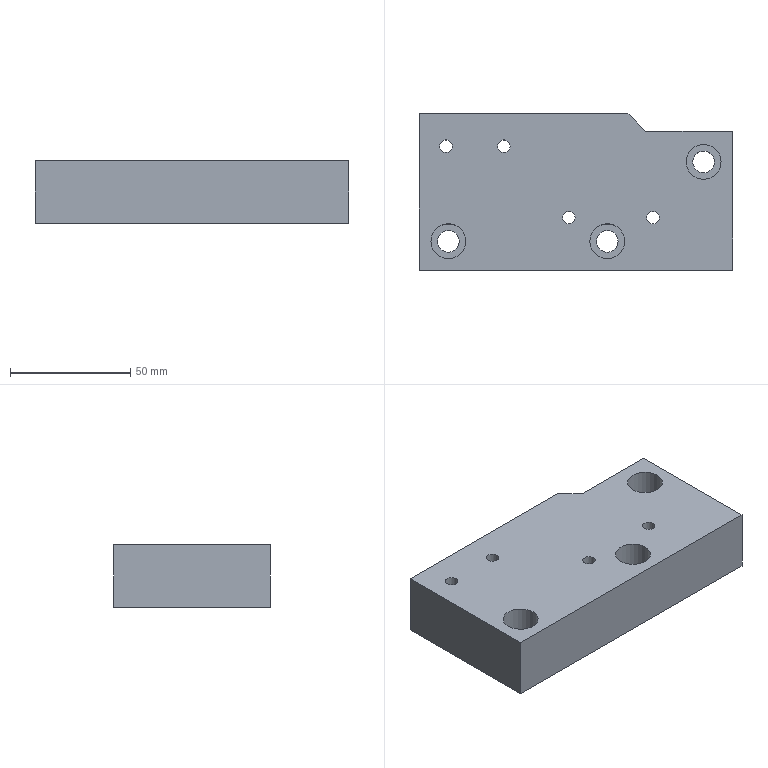Part | STEP file | lll_id678_x_t | 1 solid | 21 faces | box 130 x 65 x 26 mm | volume 201593 mm3 | plane 11 | cylinder 10 | commonest cylinder face diameters 5.206 x4 9.009 x3 14.508 x3
STEP:
#1=CARTESIAN_POINT('',(321.902,-180.325,-12.));
#2=VERTEX_POINT('',#1);
#3=CARTESIAN_POINT('',(324.505,-180.325,-12.));
#4=DIRECTION('',(0.,0.,-1.));
#5=DIRECTION('',(-1.,0.,0.));
#6=AXIS2_PLACEMENT_3D('',#3,#4,#5);
#7=CIRCLE('',#6,2.603);
#8=EDGE_CURVE('',#2,#2,#7,.T.);
#9=ORIENTED_EDGE('',*,*,#8,.T.);
#10=EDGE_LOOP('',(#9));
#11=FACE_BOUND('',#10,.T.);
#12=CARTESIAN_POINT('',(356.42,-144.5,-12.));
#13=VERTEX_POINT('',#12);
#14=CARTESIAN_POINT('',(349.095,-137.175,-12.));
#15=VERTEX_POINT('',#14);
#16=CARTESIAN_POINT('',(367.15,-155.231,-12.));
#17=DIRECTION('',(-0.7071,0.7071,0.));
#18=VECTOR('',#17,1.);
#19=LINE('',#16,#18);
#20=EDGE_CURVE('',#13,#15,#19,.T.);
#21=ORIENTED_EDGE('',*,*,#20,.T.);
#22=CARTESIAN_POINT('',(262.505,-137.175,-12.));
#23=VERTEX_POINT('',#22);
#24=CARTESIAN_POINT('',(317.505,-137.175,-12.));
#25=DIRECTION('',(-1.,0.,0.));
#26=VECTOR('',#25,1.);
#27=LINE('',#24,#26);
#28=EDGE_CURVE('',#15,#23,#27,.T.);
#29=ORIENTED_EDGE('',*,*,#28,.T.);
#30=CARTESIAN_POINT('',(262.505,-202.175,-12.));
#31=VERTEX_POINT('',#30);
#32=CARTESIAN_POINT('',(262.505,-159.675,-12.));
#33=DIRECTION('',(0.,-1.,0.));
#34=VECTOR('',#33,1.);
#35=LINE('',#32,#34);
#36=EDGE_CURVE('',#23,#31,#35,.T.);
#37=ORIENTED_EDGE('',*,*,#36,.T.);
#38=CARTESIAN_POINT('',(392.505,-202.175,-12.));
#39=VERTEX_POINT('',#38);
#40=CARTESIAN_POINT('',(317.505,-202.175,-12.));
#41=DIRECTION('',(1.,0.,0.));
#42=VECTOR('',#41,1.);
#43=LINE('',#40,#42);
#44=EDGE_CURVE('',#31,#39,#43,.T.);
#45=ORIENTED_EDGE('',*,*,#44,.T.);
#46=CARTESIAN_POINT('',(392.505,-144.5,-12.));
#47=VERTEX_POINT('',#46);
#48=CARTESIAN_POINT('',(392.505,-159.675,-12.));
#49=DIRECTION('',(0.,1.,0.));
#50=VECTOR('',#49,1.);
#51=LINE('',#48,#50);
#52=EDGE_CURVE('',#39,#47,#51,.T.);
#53=ORIENTED_EDGE('',*,*,#52,.T.);
#54=CARTESIAN_POINT('',(317.505,-144.5,-12.));
#55=DIRECTION('',(-1.,0.,0.));
#56=VECTOR('',#55,1.);
#57=LINE('',#54,#56);
#58=EDGE_CURVE('',#47,#13,#57,.T.);
#59=ORIENTED_EDGE('',*,*,#58,.T.);
#60=EDGE_LOOP('',(#21,#29,#37,#45,#53,#59));
#61=FACE_BOUND('',#60,.T.);
#62=CARTESIAN_POINT('',(270.902,-150.675,-12.));
#63=VERTEX_POINT('',#62);
#64=CARTESIAN_POINT('',(273.505,-150.675,-12.));
#65=DIRECTION('',(0.,0.,1.));
#66=DIRECTION('',(-1.,0.,0.));
#67=AXIS2_PLACEMENT_3D('',#64,#65,#66);
#68=CIRCLE('',#67,2.603);
#69=EDGE_CURVE('',#63,#63,#68,.T.);
#70=ORIENTED_EDGE('',*,*,#69,.F.);
#71=EDGE_LOOP('',(#70));
#72=FACE_BOUND('',#71,.T.);
#73=CARTESIAN_POINT('',(333.251,-190.175,-12.));
#74=VERTEX_POINT('',#73);
#75=CARTESIAN_POINT('',(340.505,-190.175,-12.));
#76=DIRECTION('',(0.,0.,1.));
#77=DIRECTION('',(-1.,0.,0.));
#78=AXIS2_PLACEMENT_3D('',#75,#76,#77);
#79=CIRCLE('',#78,7.254);
#80=EDGE_CURVE('',#74,#74,#79,.T.);
#81=ORIENTED_EDGE('',*,*,#80,.F.);
#82=EDGE_LOOP('',(#81));
#83=FACE_BOUND('',#82,.T.);
#84=CARTESIAN_POINT('',(267.251,-190.175,-12.));
#85=VERTEX_POINT('',#84);
#86=CARTESIAN_POINT('',(274.505,-190.175,-12.));
#87=DIRECTION('',(0.,0.,1.));
#88=DIRECTION('',(-1.,0.,0.));
#89=AXIS2_PLACEMENT_3D('',#86,#87,#88);
#90=CIRCLE('',#89,7.254);
#91=EDGE_CURVE('',#85,#85,#90,.T.);
#92=ORIENTED_EDGE('',*,*,#91,.F.);
#93=EDGE_LOOP('',(#92));
#94=FACE_BOUND('',#93,.T.);
#95=CARTESIAN_POINT('',(373.251,-157.175,-12.));
#96=VERTEX_POINT('',#95);
#97=CARTESIAN_POINT('',(380.505,-157.175,-12.));
#98=DIRECTION('',(0.,0.,1.));
#99=DIRECTION('',(-1.,0.,0.));
#100=AXIS2_PLACEMENT_3D('',#97,#98,#99);
#101=CIRCLE('',#100,7.254);
#102=EDGE_CURVE('',#96,#96,#101,.T.);
#103=ORIENTED_EDGE('',*,*,#102,.F.);
#104=EDGE_LOOP('',(#103));
#105=FACE_BOUND('',#104,.T.);
#106=CARTESIAN_POINT('',(294.902,-150.675,-12.));
#107=VERTEX_POINT('',#106);
#108=CARTESIAN_POINT('',(297.505,-150.675,-12.));
#109=DIRECTION('',(0.,0.,1.));
#110=DIRECTION('',(-1.,0.,0.));
#111=AXIS2_PLACEMENT_3D('',#108,#109,#110);
#112=CIRCLE('',#111,2.603);
#113=EDGE_CURVE('',#107,#107,#112,.T.);
#114=ORIENTED_EDGE('',*,*,#113,.F.);
#115=EDGE_LOOP('',(#114));
#116=FACE_BOUND('',#115,.T.);
#117=CARTESIAN_POINT('',(356.902,-180.325,-12.));
#118=VERTEX_POINT('',#117);
#119=CARTESIAN_POINT('',(359.505,-180.325,-12.));
#120=DIRECTION('',(0.,0.,-1.));
#121=DIRECTION('',(-1.,0.,0.));
#122=AXIS2_PLACEMENT_3D('',#119,#120,#121);
#123=CIRCLE('',#122,2.603);
#124=EDGE_CURVE('',#118,#118,#123,.T.);
#125=ORIENTED_EDGE('',*,*,#124,.T.);
#126=EDGE_LOOP('',(#125));
#127=FACE_BOUND('',#126,.T.);
#128=CARTESIAN_POINT('',(317.505,-159.675,-12.));
#129=DIRECTION('',(0.,0.,1.));
#130=DIRECTION('',(-1.,0.,0.));
#131=AXIS2_PLACEMENT_3D('',#128,#129,#130);
#132=PLANE('',#131);
#133=ADVANCED_FACE('',(#11,#61,#72,#83,#94,#105,#116,#127),#132,.T.);
#134=CARTESIAN_POINT('',(262.505,-137.175,-38.));
#135=VERTEX_POINT('',#134);
#136=CARTESIAN_POINT('',(349.095,-137.175,-38.));
#137=VERTEX_POINT('',#136);
#138=CARTESIAN_POINT('',(317.505,-137.175,-38.));
#139=DIRECTION('',(1.,0.,0.));
#140=VECTOR('',#139,1.);
#141=LINE('',#138,#140);
#142=EDGE_CURVE('',#135,#137,#141,.T.);
#143=ORIENTED_EDGE('',*,*,#142,.F.);
#144=CARTESIAN_POINT('',(262.505,-137.175,-38.));
#145=DIRECTION('',(0.,0.,1.));
#146=VECTOR('',#145,1.);
#147=LINE('',#144,#146);
#148=EDGE_CURVE('',#135,#23,#147,.T.);
#149=ORIENTED_EDGE('',*,*,#148,.T.);
#150=ORIENTED_EDGE('',*,*,#28,.F.);
#151=CARTESIAN_POINT('',(349.095,-137.175,-38.));
#152=DIRECTION('',(0.,0.,-1.));
#153=VECTOR('',#152,1.);
#154=LINE('',#151,#153);
#155=EDGE_CURVE('',#15,#137,#154,.T.);
#156=ORIENTED_EDGE('',*,*,#155,.T.);
#157=EDGE_LOOP('',(#143,#149,#150,#156));
#158=FACE_OUTER_BOUND('',#157,.T.);
#159=CARTESIAN_POINT('',(317.505,-137.175,-38.));
#160=DIRECTION('',(0.,1.,0.));
#161=DIRECTION('',(0.,0.,1.));
#162=AXIS2_PLACEMENT_3D('',#159,#160,#161);
#163=PLANE('',#162);
#164=ADVANCED_FACE('',(#158),#163,.T.);
#165=ORIENTED_EDGE('',*,*,#148,.F.);
#166=CARTESIAN_POINT('',(262.505,-202.175,-38.));
#167=VERTEX_POINT('',#166);
#168=CARTESIAN_POINT('',(262.505,-159.675,-38.));
#169=DIRECTION('',(0.,1.,0.));
#170=VECTOR('',#169,1.);
#171=LINE('',#168,#170);
#172=EDGE_CURVE('',#167,#135,#171,.T.);
#173=ORIENTED_EDGE('',*,*,#172,.F.);
#174=CARTESIAN_POINT('',(262.505,-202.175,-38.));
#175=DIRECTION('',(0.,0.,1.));
#176=VECTOR('',#175,1.);
#177=LINE('',#174,#176);
#178=EDGE_CURVE('',#167,#31,#177,.T.);
#179=ORIENTED_EDGE('',*,*,#178,.T.);
#180=ORIENTED_EDGE('',*,*,#36,.F.);
#181=EDGE_LOOP('',(#165,#173,#179,#180));
#182=FACE_OUTER_BOUND('',#181,.T.);
#183=CARTESIAN_POINT('',(262.505,-159.675,-38.));
#184=DIRECTION('',(-1.,0.,0.));
#185=DIRECTION('',(0.,0.,-1.));
#186=AXIS2_PLACEMENT_3D('',#183,#184,#185);
#187=PLANE('',#186);
#188=ADVANCED_FACE('',(#182),#187,.T.);
#189=ORIENTED_EDGE('',*,*,#178,.F.);
#190=CARTESIAN_POINT('',(392.505,-202.175,-38.));
#191=VERTEX_POINT('',#190);
#192=CARTESIAN_POINT('',(317.505,-202.175,-38.));
#193=DIRECTION('',(-1.,0.,0.));
#194=VECTOR('',#193,1.);
#195=LINE('',#192,#194);
#196=EDGE_CURVE('',#191,#167,#195,.T.);
#197=ORIENTED_EDGE('',*,*,#196,.F.);
#198=CARTESIAN_POINT('',(392.505,-202.175,-38.));
#199=DIRECTION('',(0.,0.,1.));
#200=VECTOR('',#199,1.);
#201=LINE('',#198,#200);
#202=EDGE_CURVE('',#191,#39,#201,.T.);
#203=ORIENTED_EDGE('',*,*,#202,.T.);
#204=ORIENTED_EDGE('',*,*,#44,.F.);
#205=EDGE_LOOP('',(#189,#197,#203,#204));
#206=FACE_OUTER_BOUND('',#205,.T.);
#207=CARTESIAN_POINT('',(317.505,-202.175,-38.));
#208=DIRECTION('',(0.,-1.,0.));
#209=DIRECTION('',(0.,0.,-1.));
#210=AXIS2_PLACEMENT_3D('',#207,#208,#209);
#211=PLANE('',#210);
#212=ADVANCED_FACE('',(#206),#211,.T.);
#213=CARTESIAN_POINT('',(356.902,-180.325,-38.));
#214=VERTEX_POINT('',#213);
#215=CARTESIAN_POINT('',(359.505,-180.325,-38.));
#216=DIRECTION('',(0.,0.,-1.));
#217=DIRECTION('',(-1.,0.,0.));
#218=AXIS2_PLACEMENT_3D('',#215,#216,#217);
#219=CIRCLE('',#218,2.603);
#220=EDGE_CURVE('',#214,#214,#219,.T.);
#221=ORIENTED_EDGE('',*,*,#220,.F.);
#222=EDGE_LOOP('',(#221));
#223=FACE_BOUND('',#222,.T.);
#224=CARTESIAN_POINT('',(321.902,-180.325,-38.));
#225=VERTEX_POINT('',#224);
#226=CARTESIAN_POINT('',(324.505,-180.325,-38.));
#227=DIRECTION('',(0.,0.,-1.));
#228=DIRECTION('',(-1.,0.,0.));
#229=AXIS2_PLACEMENT_3D('',#226,#227,#228);
#230=CIRCLE('',#229,2.603);
#231=EDGE_CURVE('',#225,#225,#230,.T.);
#232=ORIENTED_EDGE('',*,*,#231,.F.);
#233=EDGE_LOOP('',(#232));
#234=FACE_BOUND('',#233,.T.);
#235=CARTESIAN_POINT('',(356.42,-144.5,-38.));
#236=VERTEX_POINT('',#235);
#237=CARTESIAN_POINT('',(392.505,-144.5,-38.));
#238=VERTEX_POINT('',#237);
#239=CARTESIAN_POINT('',(317.505,-144.5,-38.));
#240=DIRECTION('',(1.,0.,0.));
#241=VECTOR('',#240,1.);
#242=LINE('',#239,#241);
#243=EDGE_CURVE('',#236,#238,#242,.T.);
#244=ORIENTED_EDGE('',*,*,#243,.T.);
#245=CARTESIAN_POINT('',(392.505,-159.675,-38.));
#246=DIRECTION('',(0.,-1.,0.));
#247=VECTOR('',#246,1.);
#248=LINE('',#245,#247);
#249=EDGE_CURVE('',#238,#191,#248,.T.);
#250=ORIENTED_EDGE('',*,*,#249,.T.);
#251=ORIENTED_EDGE('',*,*,#196,.T.);
#252=ORIENTED_EDGE('',*,*,#172,.T.);
#253=ORIENTED_EDGE('',*,*,#142,.T.);
#254=CARTESIAN_POINT('',(335.56,-123.641,-38.));
#255=DIRECTION('',(-0.7071,0.7071,0.));
#256=VECTOR('',#255,1.);
#257=LINE('',#254,#256);
#258=EDGE_CURVE('',#236,#137,#257,.T.);
#259=ORIENTED_EDGE('',*,*,#258,.F.);
#260=EDGE_LOOP('',(#244,#250,#251,#252,#253,#259));
#261=FACE_BOUND('',#260,.T.);
#262=CARTESIAN_POINT('',(294.902,-150.675,-38.));
#263=VERTEX_POINT('',#262);
#264=CARTESIAN_POINT('',(297.505,-150.675,-38.));
#265=DIRECTION('',(0.,0.,1.));
#266=DIRECTION('',(-1.,0.,0.));
#267=AXIS2_PLACEMENT_3D('',#264,#265,#266);
#268=CIRCLE('',#267,2.603);
#269=EDGE_CURVE('',#263,#263,#268,.T.);
#270=ORIENTED_EDGE('',*,*,#269,.T.);
#271=EDGE_LOOP('',(#270));
#272=FACE_BOUND('',#271,.T.);
#273=CARTESIAN_POINT('',(270.902,-150.675,-38.));
#274=VERTEX_POINT('',#273);
#275=CARTESIAN_POINT('',(273.505,-150.675,-38.));
#276=DIRECTION('',(0.,0.,1.));
#277=DIRECTION('',(-1.,0.,0.));
#278=AXIS2_PLACEMENT_3D('',#275,#276,#277);
#279=CIRCLE('',#278,2.603);
#280=EDGE_CURVE('',#274,#274,#279,.T.);
#281=ORIENTED_EDGE('',*,*,#280,.T.);
#282=EDGE_LOOP('',(#281));
#283=FACE_BOUND('',#282,.T.);
#284=CARTESIAN_POINT('',(376.,-157.175,-38.));
#285=VERTEX_POINT('',#284);
#286=CARTESIAN_POINT('',(380.505,-157.175,-38.));
#287=DIRECTION('',(0.,0.,1.));
#288=DIRECTION('',(-1.,0.,0.));
#289=AXIS2_PLACEMENT_3D('',#286,#287,#288);
#290=CIRCLE('',#289,4.505);
#291=EDGE_CURVE('',#285,#285,#290,.T.);
#292=ORIENTED_EDGE('',*,*,#291,.T.);
#293=EDGE_LOOP('',(#292));
#294=FACE_BOUND('',#293,.T.);
#295=CARTESIAN_POINT('',(336.,-190.175,-38.));
#296=VERTEX_POINT('',#295);
#297=CARTESIAN_POINT('',(340.505,-190.175,-38.));
#298=DIRECTION('',(0.,0.,1.));
#299=DIRECTION('',(-1.,0.,0.));
#300=AXIS2_PLACEMENT_3D('',#297,#298,#299);
#301=CIRCLE('',#300,4.505);
#302=EDGE_CURVE('',#296,#296,#301,.T.);
#303=ORIENTED_EDGE('',*,*,#302,.T.);
#304=EDGE_LOOP('',(#303));
#305=FACE_BOUND('',#304,.T.);
#306=CARTESIAN_POINT('',(270.,-190.175,-38.));
#307=VERTEX_POINT('',#306);
#308=CARTESIAN_POINT('',(274.505,-190.175,-38.));
#309=DIRECTION('',(0.,0.,1.));
#310=DIRECTION('',(-1.,0.,0.));
#311=AXIS2_PLACEMENT_3D('',#308,#309,#310);
#312=CIRCLE('',#311,4.505);
#313=EDGE_CURVE('',#307,#307,#312,.T.);
#314=ORIENTED_EDGE('',*,*,#313,.T.);
#315=EDGE_LOOP('',(#314));
#316=FACE_BOUND('',#315,.T.);
#317=CARTESIAN_POINT('',(317.505,-159.675,-38.));
#318=DIRECTION('',(0.,0.,-1.));
#319=DIRECTION('',(1.,0.,0.));
#320=AXIS2_PLACEMENT_3D('',#317,#318,#319);
#321=PLANE('',#320);
#322=ADVANCED_FACE('',(#223,#234,#261,#272,#283,#294,#305,#316),#321,.T.);
#323=CARTESIAN_POINT('',(392.505,-144.5,-38.));
#324=DIRECTION('',(0.,0.,1.));
#325=VECTOR('',#324,1.);
#326=LINE('',#323,#325);
#327=EDGE_CURVE('',#238,#47,#326,.T.);
#328=ORIENTED_EDGE('',*,*,#327,.T.);
#329=ORIENTED_EDGE('',*,*,#52,.F.);
#330=ORIENTED_EDGE('',*,*,#202,.F.);
#331=ORIENTED_EDGE('',*,*,#249,.F.);
#332=EDGE_LOOP('',(#328,#329,#330,#331));
#333=FACE_OUTER_BOUND('',#332,.T.);
#334=CARTESIAN_POINT('',(392.505,-159.675,-38.));
#335=DIRECTION('',(1.,0.,0.));
#336=DIRECTION('',(0.,0.,1.));
#337=AXIS2_PLACEMENT_3D('',#334,#335,#336);
#338=PLANE('',#337);
#339=ADVANCED_FACE('',(#333),#338,.T.);
#340=ORIENTED_EDGE('',*,*,#313,.F.);
#341=EDGE_LOOP('',(#340));
#342=FACE_BOUND('',#341,.T.);
#343=CARTESIAN_POINT('',(270.,-190.175,-23.));
#344=VERTEX_POINT('',#343);
#345=CARTESIAN_POINT('',(274.505,-190.175,-23.));
#346=DIRECTION('',(0.,0.,1.));
#347=DIRECTION('',(-1.,0.,0.));
#348=AXIS2_PLACEMENT_3D('',#345,#346,#347);
#349=CIRCLE('',#348,4.505);
#350=EDGE_CURVE('',#344,#344,#349,.T.);
#351=ORIENTED_EDGE('',*,*,#350,.T.);
#352=EDGE_LOOP('',(#351));
#353=FACE_BOUND('',#352,.T.);
#354=CARTESIAN_POINT('',(274.505,-190.175,-10.));
#355=DIRECTION('',(0.,0.,-1.));
#356=DIRECTION('',(1.,0.,0.));
#357=AXIS2_PLACEMENT_3D('',#354,#355,#356);
#358=CYLINDRICAL_SURFACE('',#357,4.505);
#359=ADVANCED_FACE('',(#342,#353),#358,.F.);
#360=ORIENTED_EDGE('',*,*,#350,.F.);
#361=EDGE_LOOP('',(#360));
#362=FACE_BOUND('',#361,.T.);
#363=CARTESIAN_POINT('',(267.251,-190.175,-23.));
#364=VERTEX_POINT('',#363);
#365=CARTESIAN_POINT('',(274.505,-190.175,-23.));
#366=DIRECTION('',(0.,0.,1.));
#367=DIRECTION('',(-1.,0.,0.));
#368=AXIS2_PLACEMENT_3D('',#365,#366,#367);
#369=CIRCLE('',#368,7.254);
#370=EDGE_CURVE('',#364,#364,#369,.T.);
#371=ORIENTED_EDGE('',*,*,#370,.T.);
#372=EDGE_LOOP('',(#371));
#373=FACE_BOUND('',#372,.T.);
#374=CARTESIAN_POINT('',(274.505,-190.175,-23.));
#375=DIRECTION('',(0.,0.,-1.));
#376=DIRECTION('',(1.,0.,0.));
#377=AXIS2_PLACEMENT_3D('',#374,#375,#376);
#378=PLANE('',#377);
#379=ADVANCED_FACE('',(#362,#373),#378,.F.);
#380=ORIENTED_EDGE('',*,*,#370,.F.);
#381=EDGE_LOOP('',(#380));
#382=FACE_BOUND('',#381,.T.);
#383=ORIENTED_EDGE('',*,*,#91,.T.);
#384=EDGE_LOOP('',(#383));
#385=FACE_BOUND('',#384,.T.);
#386=CARTESIAN_POINT('',(274.505,-190.175,-12.));
#387=DIRECTION('',(0.,0.,-1.));
#388=DIRECTION('',(1.,0.,0.));
#389=AXIS2_PLACEMENT_3D('',#386,#387,#388);
#390=CYLINDRICAL_SURFACE('',#389,7.254);
#391=ADVANCED_FACE('',(#382,#385),#390,.F.);
#392=ORIENTED_EDGE('',*,*,#302,.F.);
#393=EDGE_LOOP('',(#392));
#394=FACE_BOUND('',#393,.T.);
#395=CARTESIAN_POINT('',(336.,-190.175,-23.));
#396=VERTEX_POINT('',#395);
#397=CARTESIAN_POINT('',(340.505,-190.175,-23.));
#398=DIRECTION('',(0.,0.,1.));
#399=DIRECTION('',(-1.,0.,0.));
#400=AXIS2_PLACEMENT_3D('',#397,#398,#399);
#401=CIRCLE('',#400,4.505);
#402=EDGE_CURVE('',#396,#396,#401,.T.);
#403=ORIENTED_EDGE('',*,*,#402,.T.);
#404=EDGE_LOOP('',(#403));
#405=FACE_BOUND('',#404,.T.);
#406=CARTESIAN_POINT('',(340.505,-190.175,-10.));
#407=DIRECTION('',(0.,0.,-1.));
#408=DIRECTION('',(1.,0.,0.));
#409=AXIS2_PLACEMENT_3D('',#406,#407,#408);
#410=CYLINDRICAL_SURFACE('',#409,4.505);
#411=ADVANCED_FACE('',(#394,#405),#410,.F.);
#412=ORIENTED_EDGE('',*,*,#402,.F.);
#413=EDGE_LOOP('',(#412));
#414=FACE_BOUND('',#413,.T.);
#415=CARTESIAN_POINT('',(333.251,-190.175,-23.));
#416=VERTEX_POINT('',#415);
#417=CARTESIAN_POINT('',(340.505,-190.175,-23.));
#418=DIRECTION('',(0.,0.,1.));
#419=DIRECTION('',(-1.,0.,0.));
#420=AXIS2_PLACEMENT_3D('',#417,#418,#419);
#421=CIRCLE('',#420,7.254);
#422=EDGE_CURVE('',#416,#416,#421,.T.);
#423=ORIENTED_EDGE('',*,*,#422,.T.);
#424=EDGE_LOOP('',(#423));
#425=FACE_BOUND('',#424,.T.);
#426=CARTESIAN_POINT('',(340.505,-190.175,-23.));
#427=DIRECTION('',(0.,0.,-1.));
#428=DIRECTION('',(1.,0.,0.));
#429=AXIS2_PLACEMENT_3D('',#426,#427,#428);
#430=PLANE('',#429);
#431=ADVANCED_FACE('',(#414,#425),#430,.F.);
#432=ORIENTED_EDGE('',*,*,#422,.F.);
#433=EDGE_LOOP('',(#432));
#434=FACE_BOUND('',#433,.T.);
#435=ORIENTED_EDGE('',*,*,#80,.T.);
#436=EDGE_LOOP('',(#435));
#437=FACE_BOUND('',#436,.T.);
#438=CARTESIAN_POINT('',(340.505,-190.175,-12.));
#439=DIRECTION('',(0.,0.,-1.));
#440=DIRECTION('',(1.,0.,0.));
#441=AXIS2_PLACEMENT_3D('',#438,#439,#440);
#442=CYLINDRICAL_SURFACE('',#441,7.254);
#443=ADVANCED_FACE('',(#434,#437),#442,.F.);
#444=ORIENTED_EDGE('',*,*,#291,.F.);
#445=EDGE_LOOP('',(#444));
#446=FACE_BOUND('',#445,.T.);
#447=CARTESIAN_POINT('',(376.,-157.175,-23.));
#448=VERTEX_POINT('',#447);
#449=CARTESIAN_POINT('',(380.505,-157.175,-23.));
#450=DIRECTION('',(0.,0.,1.));
#451=DIRECTION('',(-1.,0.,0.));
#452=AXIS2_PLACEMENT_3D('',#449,#450,#451);
#453=CIRCLE('',#452,4.505);
#454=EDGE_CURVE('',#448,#448,#453,.T.);
#455=ORIENTED_EDGE('',*,*,#454,.T.);
#456=EDGE_LOOP('',(#455));
#457=FACE_BOUND('',#456,.T.);
#458=CARTESIAN_POINT('',(380.505,-157.175,-10.));
#459=DIRECTION('',(0.,0.,-1.));
#460=DIRECTION('',(1.,0.,0.));
#461=AXIS2_PLACEMENT_3D('',#458,#459,#460);
#462=CYLINDRICAL_SURFACE('',#461,4.505);
#463=ADVANCED_FACE('',(#446,#457),#462,.F.);
#464=ORIENTED_EDGE('',*,*,#454,.F.);
#465=EDGE_LOOP('',(#464));
#466=FACE_BOUND('',#465,.T.);
#467=CARTESIAN_POINT('',(373.251,-157.175,-23.));
#468=VERTEX_POINT('',#467);
#469=CARTESIAN_POINT('',(380.505,-157.175,-23.));
#470=DIRECTION('',(0.,0.,1.));
#471=DIRECTION('',(-1.,0.,0.));
#472=AXIS2_PLACEMENT_3D('',#469,#470,#471);
#473=CIRCLE('',#472,7.254);
#474=EDGE_CURVE('',#468,#468,#473,.T.);
#475=ORIENTED_EDGE('',*,*,#474,.T.);
#476=EDGE_LOOP('',(#475));
#477=FACE_BOUND('',#476,.T.);
#478=CARTESIAN_POINT('',(380.505,-157.175,-23.));
#479=DIRECTION('',(0.,0.,-1.));
#480=DIRECTION('',(1.,0.,0.));
#481=AXIS2_PLACEMENT_3D('',#478,#479,#480);
#482=PLANE('',#481);
#483=ADVANCED_FACE('',(#466,#477),#482,.F.);
#484=ORIENTED_EDGE('',*,*,#474,.F.);
#485=EDGE_LOOP('',(#484));
#486=FACE_BOUND('',#485,.T.);
#487=ORIENTED_EDGE('',*,*,#102,.T.);
#488=EDGE_LOOP('',(#487));
#489=FACE_BOUND('',#488,.T.);
#490=CARTESIAN_POINT('',(380.505,-157.175,-12.));
#491=DIRECTION('',(0.,0.,-1.));
#492=DIRECTION('',(1.,0.,0.));
#493=AXIS2_PLACEMENT_3D('',#490,#491,#492);
#494=CYLINDRICAL_SURFACE('',#493,7.254);
#495=ADVANCED_FACE('',(#486,#489),#494,.F.);
#496=ORIENTED_EDGE('',*,*,#280,.F.);
#497=EDGE_LOOP('',(#496));
#498=FACE_BOUND('',#497,.T.);
#499=ORIENTED_EDGE('',*,*,#69,.T.);
#500=EDGE_LOOP('',(#499));
#501=FACE_BOUND('',#500,.T.);
#502=CARTESIAN_POINT('',(273.505,-150.675,-12.));
#503=DIRECTION('',(0.,0.,-1.));
#504=DIRECTION('',(1.,0.,0.));
#505=AXIS2_PLACEMENT_3D('',#502,#503,#504);
#506=CYLINDRICAL_SURFACE('',#505,2.603);
#507=ADVANCED_FACE('',(#498,#501),#506,.F.);
#508=ORIENTED_EDGE('',*,*,#269,.F.);
#509=EDGE_LOOP('',(#508));
#510=FACE_BOUND('',#509,.T.);
#511=ORIENTED_EDGE('',*,*,#113,.T.);
#512=EDGE_LOOP('',(#511));
#513=FACE_BOUND('',#512,.T.);
#514=CARTESIAN_POINT('',(297.505,-150.675,-12.));
#515=DIRECTION('',(0.,0.,-1.));
#516=DIRECTION('',(1.,0.,0.));
#517=AXIS2_PLACEMENT_3D('',#514,#515,#516);
#518=CYLINDRICAL_SURFACE('',#517,2.603);
#519=ADVANCED_FACE('',(#510,#513),#518,.F.);
#520=ORIENTED_EDGE('',*,*,#258,.T.);
#521=ORIENTED_EDGE('',*,*,#155,.F.);
#522=ORIENTED_EDGE('',*,*,#20,.F.);
#523=CARTESIAN_POINT('',(356.42,-144.5,-20.));
#524=DIRECTION('',(0.,0.,-1.));
#525=VECTOR('',#524,1.);
#526=LINE('',#523,#525);
#527=EDGE_CURVE('',#13,#236,#526,.T.);
#528=ORIENTED_EDGE('',*,*,#527,.T.);
#529=EDGE_LOOP('',(#520,#521,#522,#528));
#530=FACE_OUTER_BOUND('',#529,.T.);
#531=CARTESIAN_POINT('',(335.56,-123.641,-20.));
#532=DIRECTION('',(-0.7071,-0.7071,0.));
#533=DIRECTION('',(0.,0.,-1.));
#534=AXIS2_PLACEMENT_3D('',#531,#532,#533);
#535=PLANE('',#534);
#536=ADVANCED_FACE('',(#530),#535,.F.);
#537=ORIENTED_EDGE('',*,*,#58,.F.);
#538=ORIENTED_EDGE('',*,*,#327,.F.);
#539=ORIENTED_EDGE('',*,*,#243,.F.);
#540=ORIENTED_EDGE('',*,*,#527,.F.);
#541=EDGE_LOOP('',(#537,#538,#539,#540));
#542=FACE_OUTER_BOUND('',#541,.T.);
#543=CARTESIAN_POINT('',(383.42,-144.5,-20.));
#544=DIRECTION('',(0.,-1.,0.));
#545=DIRECTION('',(0.,0.,-1.));
#546=AXIS2_PLACEMENT_3D('',#543,#544,#545);
#547=PLANE('',#546);
#548=ADVANCED_FACE('',(#542),#547,.F.);
#549=ORIENTED_EDGE('',*,*,#231,.T.);
#550=EDGE_LOOP('',(#549));
#551=FACE_BOUND('',#550,.T.);
#552=ORIENTED_EDGE('',*,*,#8,.F.);
#553=EDGE_LOOP('',(#552));
#554=FACE_BOUND('',#553,.T.);
#555=CARTESIAN_POINT('',(324.505,-180.325,-12.));
#556=DIRECTION('',(0.,0.,-1.));
#557=DIRECTION('',(1.,0.,0.));
#558=AXIS2_PLACEMENT_3D('',#555,#556,#557);
#559=CYLINDRICAL_SURFACE('',#558,2.603);
#560=ADVANCED_FACE('',(#551,#554),#559,.F.);
#561=ORIENTED_EDGE('',*,*,#220,.T.);
#562=EDGE_LOOP('',(#561));
#563=FACE_BOUND('',#562,.T.);
#564=ORIENTED_EDGE('',*,*,#124,.F.);
#565=EDGE_LOOP('',(#564));
#566=FACE_BOUND('',#565,.T.);
#567=CARTESIAN_POINT('',(359.505,-180.325,-12.));
#568=DIRECTION('',(0.,0.,-1.));
#569=DIRECTION('',(1.,0.,0.));
#570=AXIS2_PLACEMENT_3D('',#567,#568,#569);
#571=CYLINDRICAL_SURFACE('',#570,2.603);
#572=ADVANCED_FACE('',(#563,#566),#571,.F.);
#573=CLOSED_SHELL('',(#133,#164,#188,#212,#322,#339,#359,#379,#391,#411,#431,#443,#463,#483,#495,#507,#519,#536,#548,#560,#572));
#574=MANIFOLD_SOLID_BREP('',#573);
#575=(LENGTH_UNIT()NAMED_UNIT(*)SI_UNIT(.MILLI.,.METRE.));
#576=UNCERTAINTY_MEASURE_WITH_UNIT(LENGTH_MEASURE(0.00002),#575,'','');
#577=(NAMED_UNIT(*)PLANE_ANGLE_UNIT()SI_UNIT($,.RADIAN.));
#578=PLANE_ANGLE_MEASURE_WITH_UNIT(PLANE_ANGLE_MEASURE(0.01745),#577);
#579=DIMENSIONAL_EXPONENTS(0.,0.,0.,0.,0.,0.,0.);
#580=(CONVERSION_BASED_UNIT('DEGREE',#578)NAMED_UNIT(#579)PLANE_ANGLE_UNIT());
#581=(NAMED_UNIT(*)SI_UNIT($,.STERADIAN.)SOLID_ANGLE_UNIT());
#582=(GEOMETRIC_REPRESENTATION_CONTEXT(3)GLOBAL_UNCERTAINTY_ASSIGNED_CONTEXT((#576))GLOBAL_UNIT_ASSIGNED_CONTEXT((#575,#580,#581))REPRESENTATION_CONTEXT('',''));
#583=ADVANCED_BREP_SHAPE_REPRESENTATION('',(#574),#582);